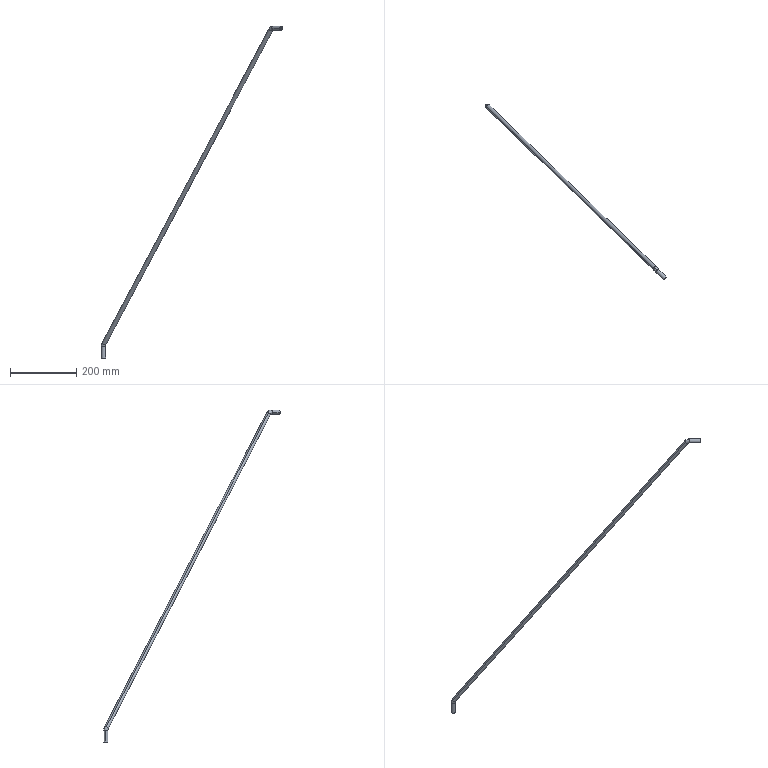Part | STEP file | Tube-500X095_2^Tube_6-P01_ASSEMBLY_KOMBAJN_OWOCOWY-003V11_Tube .500in OD X .095in Wall | 1 solid | 22 faces | box 548.949 x 534.807 x 1006 mm | volume 99272 mm3 | cylinder 12 | torus 8 | plane 2 | commonest cylinder face diameters 7.874 x6 12.7 x6